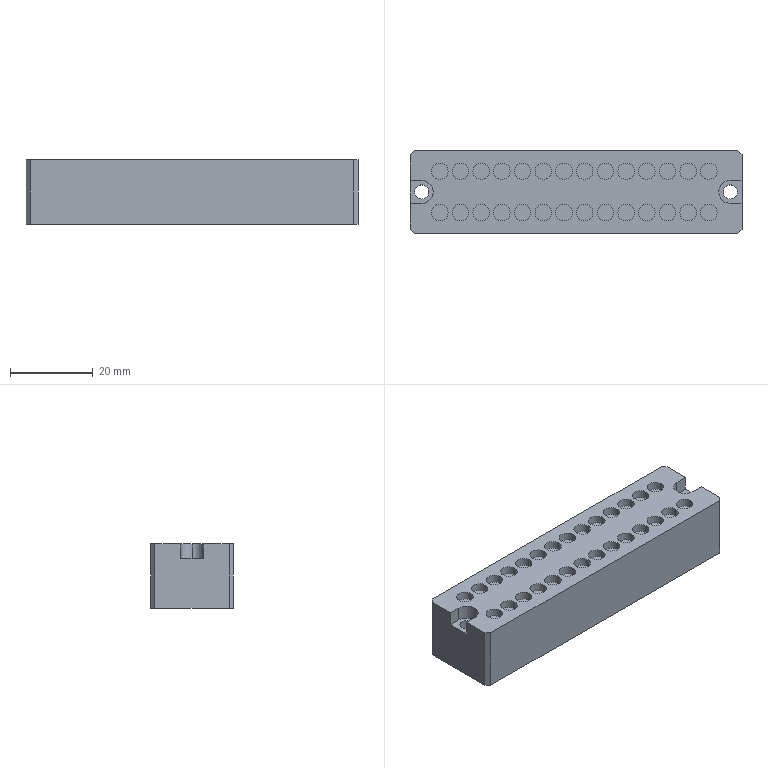Part | SolidWorks | features BaseBody 1 | 1 solid | 107 faces | box 80.2 x 20 x 15.5 mm | volume 23717 mm3 | cylinder 63 | plane 44 | commonest cylinder face diameters 4 x56 3.4 x4 5.5 x3